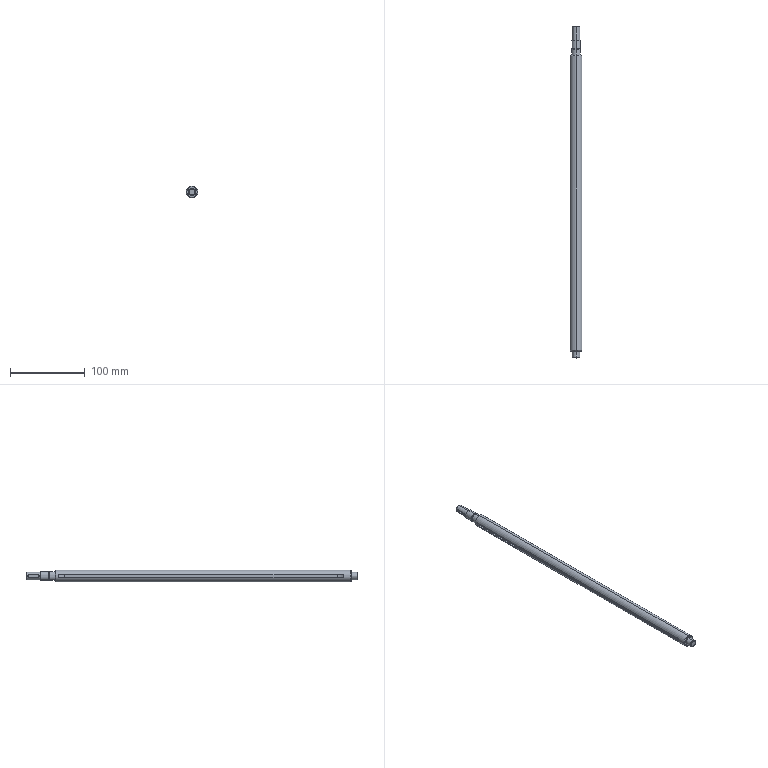Part | STEP file | 1 solid | 37 faces | box 16 x 443 x 16 mm | volume 80862 mm3 | cylinder 14 | plane 13 | cone 8 | spline 2 | commonest cylinder face diameters 10 x4 12 x4 3 x2 11.2 x2 16 x2